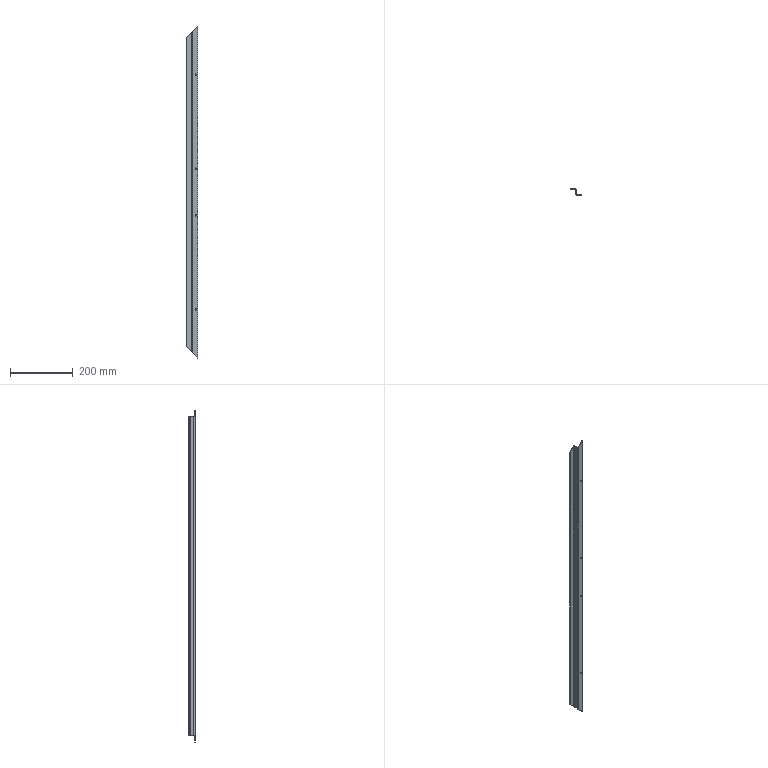Part | STEP file | SYL_0392D6J1SYL0380DJ100-648764 | 1 solid | 30 faces | box 38 x 20 x 1060 mm | volume 109009 mm3 | plane 14 | cylinder 12 | spline 4 | commonest cylinder face diameters 4.5 x8 4 x2 8 x2